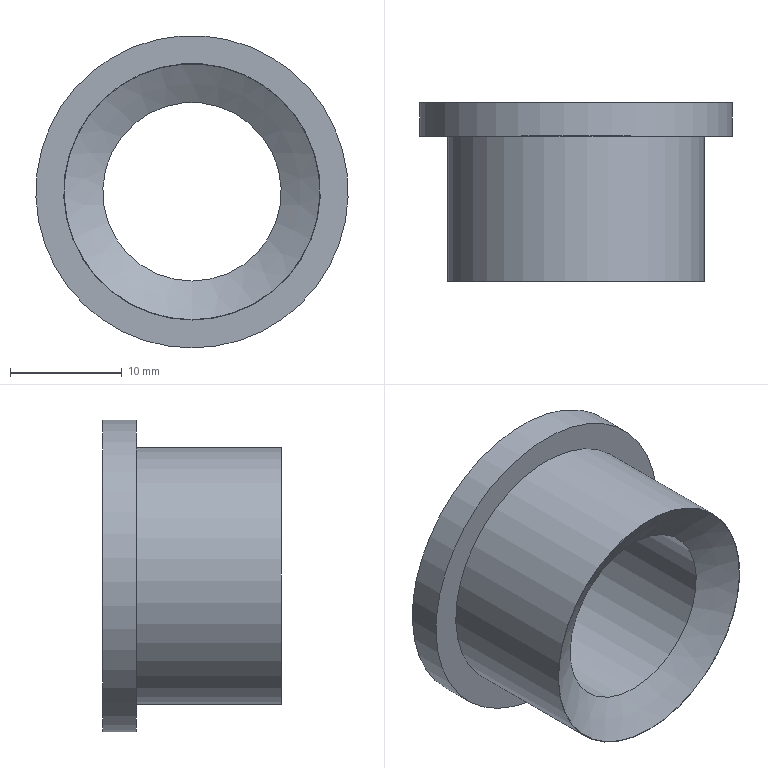Part | NX | features DATUM_CSYS 2, DATUM_PLANE 1, SKETCH 1, SWP104 1 | 1 solid | 7 faces | box 28 x 16 x 28 mm | volume 3832 mm3 | plane 3 | cylinder 3 | cone 1 | commonest cylinder face diameters 16 x1 23 x1 28 x1
STEP:
#1=CARTESIAN_POINT('',(0.,13.,-14.));
#2=VERTEX_POINT('',#1);
#3=CARTESIAN_POINT('',(0.,13.,0.));
#4=DIRECTION('',(0.,-1.,0.));
#5=DIRECTION('',(0.,0.,-1.));
#6=AXIS2_PLACEMENT_3D('',#3,#4,#5);
#7=CIRCLE('',#6,14.);
#8=EDGE_CURVE('',#2,#2,#7,.T.);
#9=ORIENTED_EDGE('',*,*,#8,.T.);
#10=EDGE_LOOP('',(#9));
#11=FACE_BOUND('',#10,.T.);
#12=CARTESIAN_POINT('',(0.,13.,-11.5));
#13=VERTEX_POINT('',#12);
#14=CARTESIAN_POINT('',(0.,13.,0.));
#15=DIRECTION('',(0.,-1.,0.));
#16=DIRECTION('',(0.,0.,-1.));
#17=AXIS2_PLACEMENT_3D('',#14,#15,#16);
#18=CIRCLE('',#17,11.5);
#19=EDGE_CURVE('',#13,#13,#18,.T.);
#20=ORIENTED_EDGE('',*,*,#19,.F.);
#21=EDGE_LOOP('',(#20));
#22=FACE_BOUND('',#21,.T.);
#23=CARTESIAN_POINT('',(0.,13.,11.5));
#24=DIRECTION('',(0.,-1.,0.));
#25=DIRECTION('',(0.,0.,-1.));
#26=AXIS2_PLACEMENT_3D('',#23,#24,#25);
#27=PLANE('',#26);
#28=ADVANCED_FACE('',(#11,#22),#27,.T.);
#29=CARTESIAN_POINT('',(0.,16.,-14.));
#30=VERTEX_POINT('',#29);
#31=CARTESIAN_POINT('',(0.,16.,0.));
#32=DIRECTION('',(0.,-1.,0.));
#33=DIRECTION('',(0.,0.,-1.));
#34=AXIS2_PLACEMENT_3D('',#31,#32,#33);
#35=CIRCLE('',#34,14.);
#36=EDGE_CURVE('',#30,#30,#35,.T.);
#37=ORIENTED_EDGE('',*,*,#36,.T.);
#38=EDGE_LOOP('',(#37));
#39=FACE_BOUND('',#38,.T.);
#40=ORIENTED_EDGE('',*,*,#8,.F.);
#41=EDGE_LOOP('',(#40));
#42=FACE_BOUND('',#41,.T.);
#43=CARTESIAN_POINT('',(0.,0.,0.));
#44=DIRECTION('',(0.,-1.,0.));
#45=DIRECTION('',(0.,0.,-1.));
#46=AXIS2_PLACEMENT_3D('',#43,#44,#45);
#47=CYLINDRICAL_SURFACE('',#46,14.);
#48=ADVANCED_FACE('',(#39,#42),#47,.T.);
#49=CARTESIAN_POINT('',(0.,16.,-8.));
#50=VERTEX_POINT('',#49);
#51=CARTESIAN_POINT('',(0.,16.,0.));
#52=DIRECTION('',(0.,-1.,0.));
#53=DIRECTION('',(0.,0.,-1.));
#54=AXIS2_PLACEMENT_3D('',#51,#52,#53);
#55=CIRCLE('',#54,8.);
#56=EDGE_CURVE('',#50,#50,#55,.T.);
#57=ORIENTED_EDGE('',*,*,#56,.T.);
#58=EDGE_LOOP('',(#57));
#59=FACE_BOUND('',#58,.T.);
#60=ORIENTED_EDGE('',*,*,#36,.F.);
#61=EDGE_LOOP('',(#60));
#62=FACE_BOUND('',#61,.T.);
#63=CARTESIAN_POINT('',(0.,16.,14.));
#64=DIRECTION('',(0.,1.,0.));
#65=DIRECTION('',(0.,0.,1.));
#66=AXIS2_PLACEMENT_3D('',#63,#64,#65);
#67=PLANE('',#66);
#68=ADVANCED_FACE('',(#59,#62),#67,.T.);
#69=CARTESIAN_POINT('',(0.,2.,-8.));
#70=VERTEX_POINT('',#69);
#71=CARTESIAN_POINT('',(0.,2.,0.));
#72=DIRECTION('',(0.,-1.,0.));
#73=DIRECTION('',(0.,0.,-1.));
#74=AXIS2_PLACEMENT_3D('',#71,#72,#73);
#75=CIRCLE('',#74,8.);
#76=EDGE_CURVE('',#70,#70,#75,.T.);
#77=ORIENTED_EDGE('',*,*,#76,.T.);
#78=EDGE_LOOP('',(#77));
#79=FACE_BOUND('',#78,.T.);
#80=ORIENTED_EDGE('',*,*,#56,.F.);
#81=EDGE_LOOP('',(#80));
#82=FACE_BOUND('',#81,.T.);
#83=CARTESIAN_POINT('',(0.,0.,0.));
#84=DIRECTION('',(0.,-1.,0.));
#85=DIRECTION('',(0.,0.,-1.));
#86=AXIS2_PLACEMENT_3D('',#83,#84,#85);
#87=CYLINDRICAL_SURFACE('',#86,8.);
#88=ADVANCED_FACE('',(#79,#82),#87,.F.);
#89=CARTESIAN_POINT('',(0.,0.,-11.464));
#90=VERTEX_POINT('',#89);
#91=CARTESIAN_POINT('',(0.,0.,0.));
#92=DIRECTION('',(0.,-1.,0.));
#93=DIRECTION('',(0.,0.,-1.));
#94=AXIS2_PLACEMENT_3D('',#91,#92,#93);
#95=CIRCLE('',#94,11.464);
#96=EDGE_CURVE('',#90,#90,#95,.T.);
#97=ORIENTED_EDGE('',*,*,#96,.T.);
#98=EDGE_LOOP('',(#97));
#99=FACE_BOUND('',#98,.T.);
#100=ORIENTED_EDGE('',*,*,#76,.F.);
#101=EDGE_LOOP('',(#100));
#102=FACE_BOUND('',#101,.T.);
#103=CARTESIAN_POINT('',(0.,2.,0.));
#104=DIRECTION('',(0.,-1.,0.));
#105=DIRECTION('',(0.,0.,-1.));
#106=AXIS2_PLACEMENT_3D('',#103,#104,#105);
#107=CONICAL_SURFACE('',#106,8.,1.047);
#108=ADVANCED_FACE('',(#99,#102),#107,.F.);
#109=CARTESIAN_POINT('',(0.,0.,-11.5));
#110=VERTEX_POINT('',#109);
#111=CARTESIAN_POINT('',(0.,0.,0.));
#112=DIRECTION('',(0.,-1.,0.));
#113=DIRECTION('',(0.,0.,-1.));
#114=AXIS2_PLACEMENT_3D('',#111,#112,#113);
#115=CIRCLE('',#114,11.5);
#116=EDGE_CURVE('',#110,#110,#115,.T.);
#117=ORIENTED_EDGE('',*,*,#116,.T.);
#118=EDGE_LOOP('',(#117));
#119=FACE_BOUND('',#118,.T.);
#120=ORIENTED_EDGE('',*,*,#96,.F.);
#121=EDGE_LOOP('',(#120));
#122=FACE_BOUND('',#121,.T.);
#123=CARTESIAN_POINT('',(0.,0.,11.464));
#124=DIRECTION('',(0.,-1.,0.));
#125=DIRECTION('',(0.,0.,-1.));
#126=AXIS2_PLACEMENT_3D('',#123,#124,#125);
#127=PLANE('',#126);
#128=ADVANCED_FACE('',(#119,#122),#127,.T.);
#129=ORIENTED_EDGE('',*,*,#19,.T.);
#130=EDGE_LOOP('',(#129));
#131=FACE_BOUND('',#130,.T.);
#132=ORIENTED_EDGE('',*,*,#116,.F.);
#133=EDGE_LOOP('',(#132));
#134=FACE_BOUND('',#133,.T.);
#135=CARTESIAN_POINT('',(0.,0.,0.));
#136=DIRECTION('',(0.,-1.,0.));
#137=DIRECTION('',(0.,0.,-1.));
#138=AXIS2_PLACEMENT_3D('',#135,#136,#137);
#139=CYLINDRICAL_SURFACE('',#138,11.5);
#140=ADVANCED_FACE('',(#131,#134),#139,.T.);
#141=CLOSED_SHELL('',(#28,#48,#68,#88,#108,#128,#140));
#142=MANIFOLD_SOLID_BREP('',#141);
#143=(LENGTH_UNIT()NAMED_UNIT(*)SI_UNIT(.MILLI.,.METRE.));
#144=UNCERTAINTY_MEASURE_WITH_UNIT(LENGTH_MEASURE(0.00001),#143,'','');
#145=(NAMED_UNIT(*)PLANE_ANGLE_UNIT()SI_UNIT($,.RADIAN.));
#146=(NAMED_UNIT(*)SI_UNIT($,.STERADIAN.)SOLID_ANGLE_UNIT());
#147=(GEOMETRIC_REPRESENTATION_CONTEXT(3)GLOBAL_UNCERTAINTY_ASSIGNED_CONTEXT((#144))GLOBAL_UNIT_ASSIGNED_CONTEXT((#143,#145,#146))REPRESENTATION_CONTEXT('',''));
#148=ADVANCED_BREP_SHAPE_REPRESENTATION('',(#142),#147);